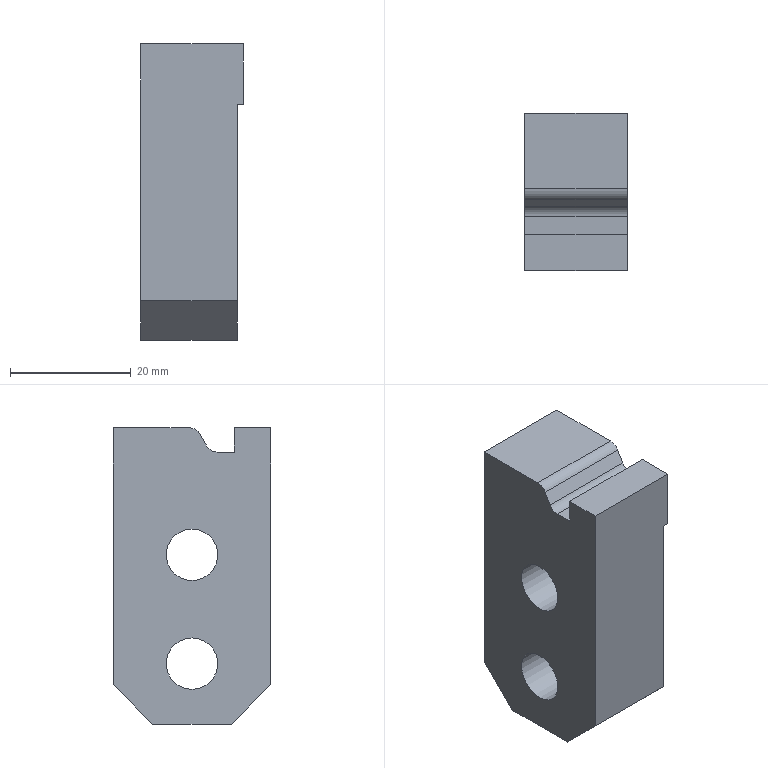Part | STEP file | gslz 2016.10.28-13_id1746_x_t | 1 solid | 22 faces | box 17 x 26 x 49 mm | volume 16052 mm3 | plane 16 | cylinder 6 | commonest cylinder face diameters 4 x2 8.5 x2 14 x2